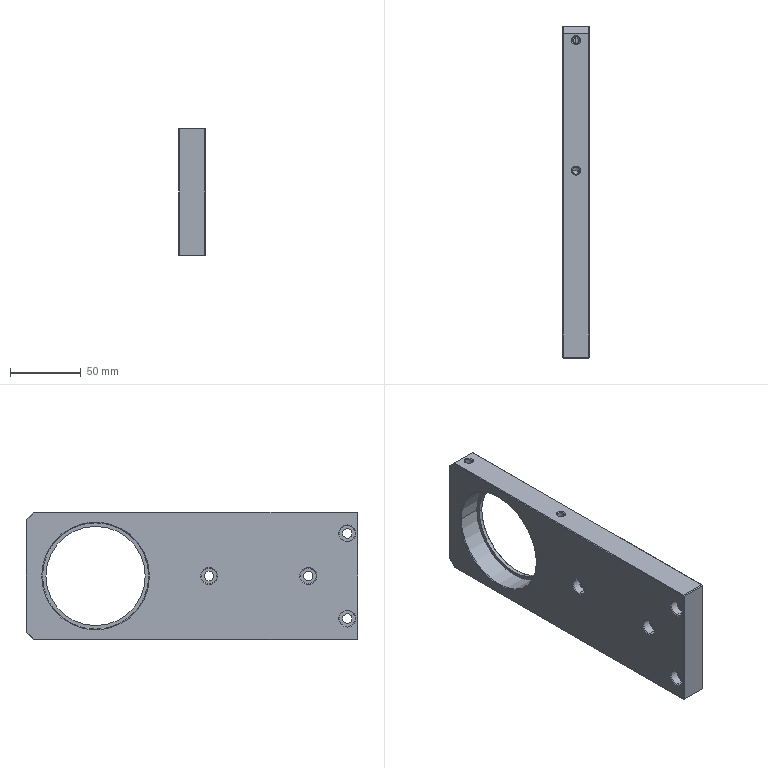Part | SolidWorks | features HoleWzd 6, Chamfer 3, ICE 3, Extrusion 1, Fillet 1, MoveFace 1 | 1 solid | 111 faces | box 19 x 234 x 90 mm | volume 311217 mm3 | cone 46 | cylinder 36 | plane 29 | commonest cylinder face diameters 5 x12 6.6 x8 11 x8 2.5 x4 70 x2 75 x2